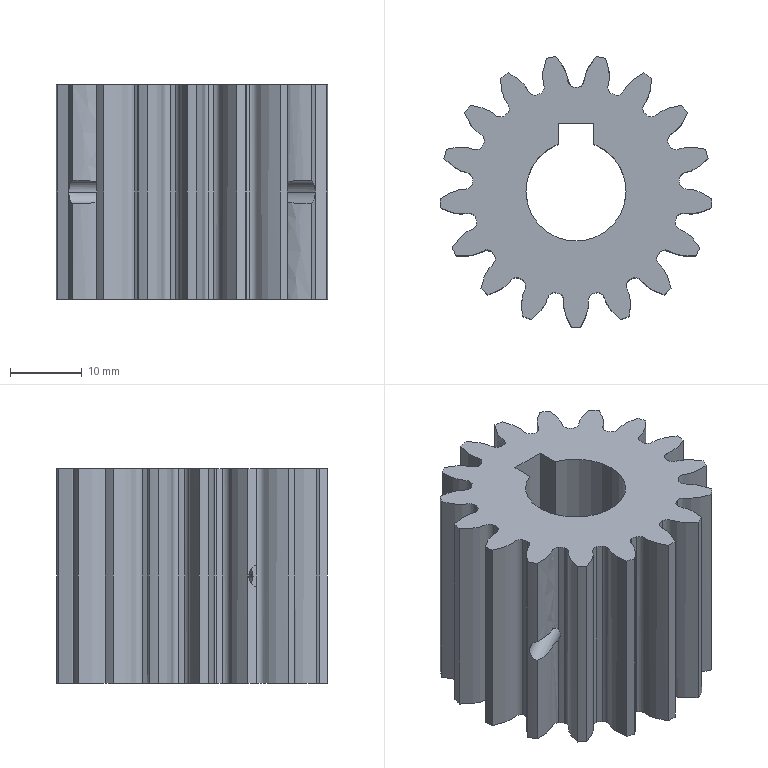Part | SolidWorks | features CirPattern 2, ICE 2, Extrusion 1, HoleWzd 1, RefAxis 1 | 1 solid | 85 faces | box 37.938 x 37.788 x 30 mm | volume 21474 mm3 | cylinder 44 | spline 36 | plane 5 | commonest cylinder face diameters 29 x18 38 x17 3.3 x6 14 x3